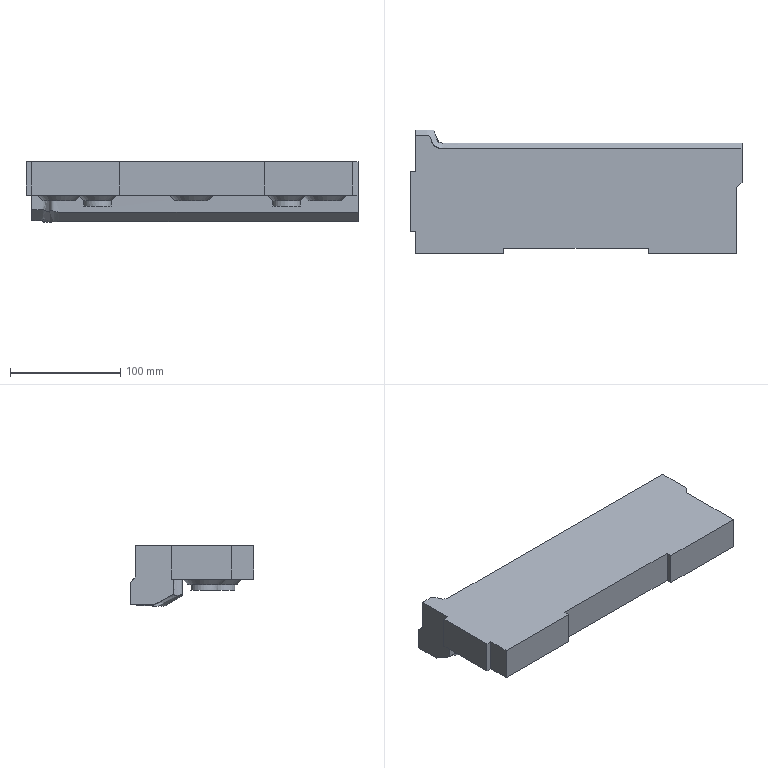Part | NX | features solid 2 | 1 solid | 34 faces | box 301.026 x 112.418 x 54.519 mm | volume 1079153 mm3 | plane 21 | spline 6 | cone 5 | cylinder 2 | commonest cylinder face diameters 25 x2